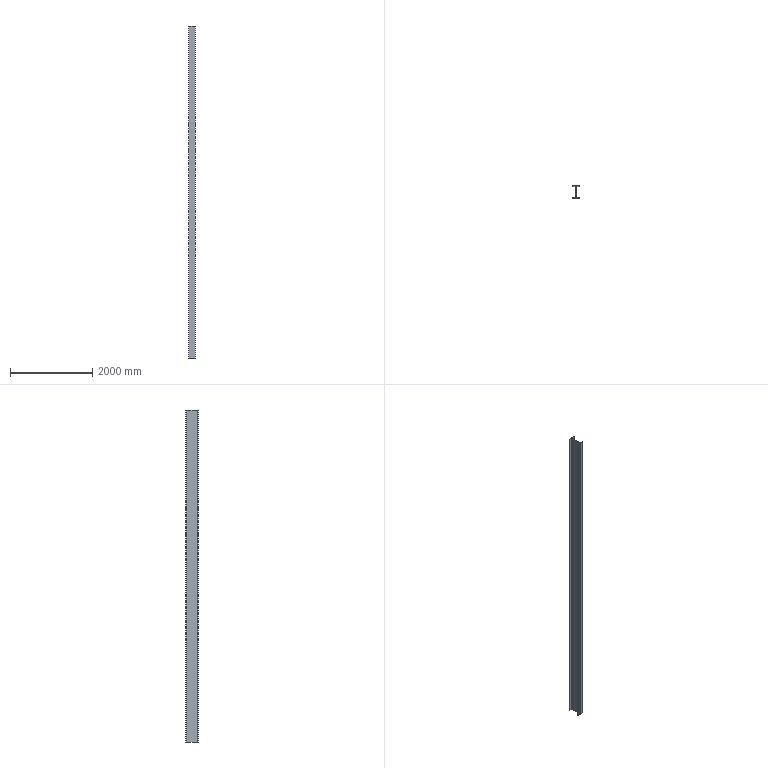Part | SolidWorks | features Extrusion 1 | 1 solid | 18 faces | box 150 x 300 x 8090 mm | volume 37845593 mm3 | plane 14 | cylinder 4 | commonest cylinder face diameters 26 x4
STEP:
#1=CARTESIAN_POINT('',(-75.,9.,0.));
#2=VERTEX_POINT('',#1);
#3=CARTESIAN_POINT('',(-75.,0.,0.));
#4=VERTEX_POINT('',#3);
#5=CARTESIAN_POINT('',(-75.,0.,0.));
#6=DIRECTION('',(0.,-1.,0.));
#7=VECTOR('',#6,1000.);
#8=LINE('',#5,#7);
#9=EDGE_CURVE('',#2,#4,#8,.T.);
#10=ORIENTED_EDGE('',*,*,#9,.T.);
#11=CARTESIAN_POINT('',(-75.,0.,8090.));
#12=VERTEX_POINT('',#11);
#13=CARTESIAN_POINT('',(-75.,0.,8090.));
#14=DIRECTION('',(0.,0.,-1.));
#15=VECTOR('',#14,1000.);
#16=LINE('',#13,#15);
#17=EDGE_CURVE('',#12,#4,#16,.T.);
#18=ORIENTED_EDGE('',*,*,#17,.F.);
#19=CARTESIAN_POINT('',(-75.,9.,8090.));
#20=VERTEX_POINT('',#19);
#21=CARTESIAN_POINT('',(-75.,0.,8090.));
#22=DIRECTION('',(0.,-1.,0.));
#23=VECTOR('',#22,1000.);
#24=LINE('',#21,#23);
#25=EDGE_CURVE('',#20,#12,#24,.T.);
#26=ORIENTED_EDGE('',*,*,#25,.F.);
#27=CARTESIAN_POINT('',(-75.,9.,8090.));
#28=DIRECTION('',(0.,0.,-1.));
#29=VECTOR('',#28,1000.);
#30=LINE('',#27,#29);
#31=EDGE_CURVE('',#20,#2,#30,.T.);
#32=ORIENTED_EDGE('',*,*,#31,.T.);
#33=EDGE_LOOP('',(#10,#18,#26,#32));
#34=FACE_OUTER_BOUND('',#33,.T.);
#35=CARTESIAN_POINT('',(-75.,0.,8090.));
#36=DIRECTION('',(1.,0.,0.));
#37=DIRECTION('',(0.,0.,-1.));
#38=AXIS2_PLACEMENT_3D('',#35,#36,#37);
#39=PLANE('',#38);
#40=ADVANCED_FACE('',(#34),#39,.F.);
#41=CARTESIAN_POINT('',(75.,0.,0.));
#42=VERTEX_POINT('',#41);
#43=CARTESIAN_POINT('',(75.,0.,0.));
#44=DIRECTION('',(1.,0.,0.));
#45=VECTOR('',#44,1000.);
#46=LINE('',#43,#45);
#47=EDGE_CURVE('',#4,#42,#46,.T.);
#48=ORIENTED_EDGE('',*,*,#47,.T.);
#49=CARTESIAN_POINT('',(75.,0.,8090.));
#50=VERTEX_POINT('',#49);
#51=CARTESIAN_POINT('',(75.,0.,8090.));
#52=DIRECTION('',(0.,0.,-1.));
#53=VECTOR('',#52,1000.);
#54=LINE('',#51,#53);
#55=EDGE_CURVE('',#50,#42,#54,.T.);
#56=ORIENTED_EDGE('',*,*,#55,.F.);
#57=CARTESIAN_POINT('',(75.,0.,8090.));
#58=DIRECTION('',(1.,0.,0.));
#59=VECTOR('',#58,1000.);
#60=LINE('',#57,#59);
#61=EDGE_CURVE('',#12,#50,#60,.T.);
#62=ORIENTED_EDGE('',*,*,#61,.F.);
#63=ORIENTED_EDGE('',*,*,#17,.T.);
#64=EDGE_LOOP('',(#48,#56,#62,#63));
#65=FACE_OUTER_BOUND('',#64,.T.);
#66=CARTESIAN_POINT('',(75.,0.,8090.));
#67=DIRECTION('',(0.,1.,0.));
#68=DIRECTION('',(-1.,0.,0.));
#69=AXIS2_PLACEMENT_3D('',#66,#67,#68);
#70=PLANE('',#69);
#71=ADVANCED_FACE('',(#65),#70,.F.);
#72=CARTESIAN_POINT('',(75.,9.,0.));
#73=VERTEX_POINT('',#72);
#74=CARTESIAN_POINT('',(75.,0.,0.));
#75=DIRECTION('',(0.,1.,0.));
#76=VECTOR('',#75,1000.);
#77=LINE('',#74,#76);
#78=EDGE_CURVE('',#42,#73,#77,.T.);
#79=ORIENTED_EDGE('',*,*,#78,.T.);
#80=CARTESIAN_POINT('',(75.,9.,8090.));
#81=VERTEX_POINT('',#80);
#82=CARTESIAN_POINT('',(75.,9.,8090.));
#83=DIRECTION('',(0.,0.,-1.));
#84=VECTOR('',#83,1000.);
#85=LINE('',#82,#84);
#86=EDGE_CURVE('',#81,#73,#85,.T.);
#87=ORIENTED_EDGE('',*,*,#86,.F.);
#88=CARTESIAN_POINT('',(75.,0.,8090.));
#89=DIRECTION('',(0.,1.,0.));
#90=VECTOR('',#89,1000.);
#91=LINE('',#88,#90);
#92=EDGE_CURVE('',#50,#81,#91,.T.);
#93=ORIENTED_EDGE('',*,*,#92,.F.);
#94=ORIENTED_EDGE('',*,*,#55,.T.);
#95=EDGE_LOOP('',(#79,#87,#93,#94));
#96=FACE_OUTER_BOUND('',#95,.T.);
#97=CARTESIAN_POINT('',(75.,0.,8090.));
#98=DIRECTION('',(-1.,0.,0.));
#99=DIRECTION('',(0.,0.,1.));
#100=AXIS2_PLACEMENT_3D('',#97,#98,#99);
#101=PLANE('',#100);
#102=ADVANCED_FACE('',(#96),#101,.F.);
#103=CARTESIAN_POINT('',(16.25,9.,0.));
#104=VERTEX_POINT('',#103);
#105=CARTESIAN_POINT('',(75.,9.,0.));
#106=DIRECTION('',(-1.,0.,0.));
#107=VECTOR('',#106,1000.);
#108=LINE('',#105,#107);
#109=EDGE_CURVE('',#73,#104,#108,.T.);
#110=ORIENTED_EDGE('',*,*,#109,.T.);
#111=CARTESIAN_POINT('',(16.25,9.,8090.));
#112=VERTEX_POINT('',#111);
#113=CARTESIAN_POINT('',(16.25,9.,8090.));
#114=DIRECTION('',(0.,0.,-1.));
#115=VECTOR('',#114,1000.);
#116=LINE('',#113,#115);
#117=EDGE_CURVE('',#112,#104,#116,.T.);
#118=ORIENTED_EDGE('',*,*,#117,.F.);
#119=CARTESIAN_POINT('',(75.,9.,8090.));
#120=DIRECTION('',(-1.,0.,0.));
#121=VECTOR('',#120,1000.);
#122=LINE('',#119,#121);
#123=EDGE_CURVE('',#81,#112,#122,.T.);
#124=ORIENTED_EDGE('',*,*,#123,.F.);
#125=ORIENTED_EDGE('',*,*,#86,.T.);
#126=EDGE_LOOP('',(#110,#118,#124,#125));
#127=FACE_OUTER_BOUND('',#126,.T.);
#128=CARTESIAN_POINT('',(75.,9.,8090.));
#129=DIRECTION('',(0.,-1.,0.));
#130=DIRECTION('',(1.,0.,0.));
#131=AXIS2_PLACEMENT_3D('',#128,#129,#130);
#132=PLANE('',#131);
#133=ADVANCED_FACE('',(#127),#132,.F.);
#134=CARTESIAN_POINT('',(3.25,22.,0.));
#135=VERTEX_POINT('',#134);
#136=CARTESIAN_POINT('',(16.25,22.,0.));
#137=DIRECTION('',(0.,0.,-1.));
#138=DIRECTION('',(-1.,0.,0.));
#139=AXIS2_PLACEMENT_3D('',#136,#137,#138);
#140=CIRCLE('',#139,13.);
#141=EDGE_CURVE('',#104,#135,#140,.T.);
#142=ORIENTED_EDGE('',*,*,#141,.T.);
#143=CARTESIAN_POINT('',(3.25,22.,8090.));
#144=VERTEX_POINT('',#143);
#145=CARTESIAN_POINT('',(3.25,22.,8090.));
#146=DIRECTION('',(0.,0.,-1.));
#147=VECTOR('',#146,1000.);
#148=LINE('',#145,#147);
#149=EDGE_CURVE('',#144,#135,#148,.T.);
#150=ORIENTED_EDGE('',*,*,#149,.F.);
#151=CARTESIAN_POINT('',(16.25,22.,8090.));
#152=DIRECTION('',(0.,0.,-1.));
#153=DIRECTION('',(-1.,0.,0.));
#154=AXIS2_PLACEMENT_3D('',#151,#152,#153);
#155=CIRCLE('',#154,13.);
#156=EDGE_CURVE('',#112,#144,#155,.T.);
#157=ORIENTED_EDGE('',*,*,#156,.F.);
#158=ORIENTED_EDGE('',*,*,#117,.T.);
#159=EDGE_LOOP('',(#142,#150,#157,#158));
#160=FACE_OUTER_BOUND('',#159,.T.);
#161=CARTESIAN_POINT('',(16.25,22.,8090.));
#162=DIRECTION('',(0.,0.,-1.));
#163=DIRECTION('',(-1.,0.,0.));
#164=AXIS2_PLACEMENT_3D('',#161,#162,#163);
#165=CYLINDRICAL_SURFACE('',#164,13.);
#166=ADVANCED_FACE('',(#160),#165,.F.);
#167=CARTESIAN_POINT('',(3.25,278.,0.));
#168=VERTEX_POINT('',#167);
#169=CARTESIAN_POINT('',(3.25,22.,0.));
#170=DIRECTION('',(0.,1.,0.));
#171=VECTOR('',#170,1000.);
#172=LINE('',#169,#171);
#173=EDGE_CURVE('',#135,#168,#172,.T.);
#174=ORIENTED_EDGE('',*,*,#173,.T.);
#175=CARTESIAN_POINT('',(3.25,278.,8090.));
#176=VERTEX_POINT('',#175);
#177=CARTESIAN_POINT('',(3.25,278.,8090.));
#178=DIRECTION('',(0.,0.,-1.));
#179=VECTOR('',#178,1000.);
#180=LINE('',#177,#179);
#181=EDGE_CURVE('',#176,#168,#180,.T.);
#182=ORIENTED_EDGE('',*,*,#181,.F.);
#183=CARTESIAN_POINT('',(3.25,22.,8090.));
#184=DIRECTION('',(0.,1.,0.));
#185=VECTOR('',#184,1000.);
#186=LINE('',#183,#185);
#187=EDGE_CURVE('',#144,#176,#186,.T.);
#188=ORIENTED_EDGE('',*,*,#187,.F.);
#189=ORIENTED_EDGE('',*,*,#149,.T.);
#190=EDGE_LOOP('',(#174,#182,#188,#189));
#191=FACE_OUTER_BOUND('',#190,.T.);
#192=CARTESIAN_POINT('',(3.25,22.,8090.));
#193=DIRECTION('',(-1.,0.,0.));
#194=DIRECTION('',(0.,0.,1.));
#195=AXIS2_PLACEMENT_3D('',#192,#193,#194);
#196=PLANE('',#195);
#197=ADVANCED_FACE('',(#191),#196,.F.);
#198=CARTESIAN_POINT('',(16.25,291.,0.));
#199=VERTEX_POINT('',#198);
#200=CARTESIAN_POINT('',(16.25,278.,0.));
#201=DIRECTION('',(0.,0.,-1.));
#202=DIRECTION('',(-1.,0.,0.));
#203=AXIS2_PLACEMENT_3D('',#200,#201,#202);
#204=CIRCLE('',#203,13.);
#205=EDGE_CURVE('',#168,#199,#204,.T.);
#206=ORIENTED_EDGE('',*,*,#205,.T.);
#207=CARTESIAN_POINT('',(16.25,291.,8090.));
#208=VERTEX_POINT('',#207);
#209=CARTESIAN_POINT('',(16.25,291.,8090.));
#210=DIRECTION('',(0.,0.,-1.));
#211=VECTOR('',#210,1000.);
#212=LINE('',#209,#211);
#213=EDGE_CURVE('',#208,#199,#212,.T.);
#214=ORIENTED_EDGE('',*,*,#213,.F.);
#215=CARTESIAN_POINT('',(16.25,278.,8090.));
#216=DIRECTION('',(0.,0.,-1.));
#217=DIRECTION('',(-1.,0.,0.));
#218=AXIS2_PLACEMENT_3D('',#215,#216,#217);
#219=CIRCLE('',#218,13.);
#220=EDGE_CURVE('',#176,#208,#219,.T.);
#221=ORIENTED_EDGE('',*,*,#220,.F.);
#222=ORIENTED_EDGE('',*,*,#181,.T.);
#223=EDGE_LOOP('',(#206,#214,#221,#222));
#224=FACE_OUTER_BOUND('',#223,.T.);
#225=CARTESIAN_POINT('',(16.25,278.,8090.));
#226=DIRECTION('',(0.,0.,-1.));
#227=DIRECTION('',(-1.,0.,0.));
#228=AXIS2_PLACEMENT_3D('',#225,#226,#227);
#229=CYLINDRICAL_SURFACE('',#228,13.);
#230=ADVANCED_FACE('',(#224),#229,.F.);
#231=CARTESIAN_POINT('',(75.,291.,0.));
#232=VERTEX_POINT('',#231);
#233=CARTESIAN_POINT('',(16.25,291.,0.));
#234=DIRECTION('',(1.,0.,0.));
#235=VECTOR('',#234,1000.);
#236=LINE('',#233,#235);
#237=EDGE_CURVE('',#199,#232,#236,.T.);
#238=ORIENTED_EDGE('',*,*,#237,.T.);
#239=CARTESIAN_POINT('',(75.,291.,8090.));
#240=VERTEX_POINT('',#239);
#241=CARTESIAN_POINT('',(75.,291.,8090.));
#242=DIRECTION('',(0.,0.,-1.));
#243=VECTOR('',#242,1000.);
#244=LINE('',#241,#243);
#245=EDGE_CURVE('',#240,#232,#244,.T.);
#246=ORIENTED_EDGE('',*,*,#245,.F.);
#247=CARTESIAN_POINT('',(16.25,291.,8090.));
#248=DIRECTION('',(1.,0.,0.));
#249=VECTOR('',#248,1000.);
#250=LINE('',#247,#249);
#251=EDGE_CURVE('',#208,#240,#250,.T.);
#252=ORIENTED_EDGE('',*,*,#251,.F.);
#253=ORIENTED_EDGE('',*,*,#213,.T.);
#254=EDGE_LOOP('',(#238,#246,#252,#253));
#255=FACE_OUTER_BOUND('',#254,.T.);
#256=CARTESIAN_POINT('',(16.25,291.,8090.));
#257=DIRECTION('',(0.,1.,0.));
#258=DIRECTION('',(-1.,0.,0.));
#259=AXIS2_PLACEMENT_3D('',#256,#257,#258);
#260=PLANE('',#259);
#261=ADVANCED_FACE('',(#255),#260,.F.);
#262=CARTESIAN_POINT('',(75.,300.,0.));
#263=VERTEX_POINT('',#262);
#264=CARTESIAN_POINT('',(75.,291.,0.));
#265=DIRECTION('',(0.,1.,0.));
#266=VECTOR('',#265,1000.);
#267=LINE('',#264,#266);
#268=EDGE_CURVE('',#232,#263,#267,.T.);
#269=ORIENTED_EDGE('',*,*,#268,.T.);
#270=CARTESIAN_POINT('',(75.,300.,8090.));
#271=VERTEX_POINT('',#270);
#272=CARTESIAN_POINT('',(75.,300.,8090.));
#273=DIRECTION('',(0.,0.,-1.));
#274=VECTOR('',#273,1000.);
#275=LINE('',#272,#274);
#276=EDGE_CURVE('',#271,#263,#275,.T.);
#277=ORIENTED_EDGE('',*,*,#276,.F.);
#278=CARTESIAN_POINT('',(75.,291.,8090.));
#279=DIRECTION('',(0.,1.,0.));
#280=VECTOR('',#279,1000.);
#281=LINE('',#278,#280);
#282=EDGE_CURVE('',#240,#271,#281,.T.);
#283=ORIENTED_EDGE('',*,*,#282,.F.);
#284=ORIENTED_EDGE('',*,*,#245,.T.);
#285=EDGE_LOOP('',(#269,#277,#283,#284));
#286=FACE_OUTER_BOUND('',#285,.T.);
#287=CARTESIAN_POINT('',(75.,291.,8090.));
#288=DIRECTION('',(-1.,0.,0.));
#289=DIRECTION('',(0.,-1.,0.));
#290=AXIS2_PLACEMENT_3D('',#287,#288,#289);
#291=PLANE('',#290);
#292=ADVANCED_FACE('',(#286),#291,.F.);
#293=CARTESIAN_POINT('',(-75.,300.,0.));
#294=VERTEX_POINT('',#293);
#295=CARTESIAN_POINT('',(-75.,300.,0.));
#296=DIRECTION('',(-1.,0.,0.));
#297=VECTOR('',#296,1000.);
#298=LINE('',#295,#297);
#299=EDGE_CURVE('',#263,#294,#298,.T.);
#300=ORIENTED_EDGE('',*,*,#299,.T.);
#301=CARTESIAN_POINT('',(-75.,300.,8090.));
#302=VERTEX_POINT('',#301);
#303=CARTESIAN_POINT('',(-75.,300.,8090.));
#304=DIRECTION('',(0.,0.,-1.));
#305=VECTOR('',#304,1000.);
#306=LINE('',#303,#305);
#307=EDGE_CURVE('',#302,#294,#306,.T.);
#308=ORIENTED_EDGE('',*,*,#307,.F.);
#309=CARTESIAN_POINT('',(-75.,300.,8090.));
#310=DIRECTION('',(-1.,0.,0.));
#311=VECTOR('',#310,1000.);
#312=LINE('',#309,#311);
#313=EDGE_CURVE('',#271,#302,#312,.T.);
#314=ORIENTED_EDGE('',*,*,#313,.F.);
#315=ORIENTED_EDGE('',*,*,#276,.T.);
#316=EDGE_LOOP('',(#300,#308,#314,#315));
#317=FACE_OUTER_BOUND('',#316,.T.);
#318=CARTESIAN_POINT('',(-75.,300.,8090.));
#319=DIRECTION('',(0.,-1.,0.));
#320=DIRECTION('',(0.,0.,-1.));
#321=AXIS2_PLACEMENT_3D('',#318,#319,#320);
#322=PLANE('',#321);
#323=ADVANCED_FACE('',(#317),#322,.F.);
#324=CARTESIAN_POINT('',(-75.,291.,0.));
#325=VERTEX_POINT('',#324);
#326=CARTESIAN_POINT('',(-75.,291.,0.));
#327=DIRECTION('',(0.,-1.,0.));
#328=VECTOR('',#327,1000.);
#329=LINE('',#326,#328);
#330=EDGE_CURVE('',#294,#325,#329,.T.);
#331=ORIENTED_EDGE('',*,*,#330,.T.);
#332=CARTESIAN_POINT('',(-75.,291.,8090.));
#333=VERTEX_POINT('',#332);
#334=CARTESIAN_POINT('',(-75.,291.,8090.));
#335=DIRECTION('',(0.,0.,-1.));
#336=VECTOR('',#335,1000.);
#337=LINE('',#334,#336);
#338=EDGE_CURVE('',#333,#325,#337,.T.);
#339=ORIENTED_EDGE('',*,*,#338,.F.);
#340=CARTESIAN_POINT('',(-75.,291.,8090.));
#341=DIRECTION('',(0.,-1.,0.));
#342=VECTOR('',#341,1000.);
#343=LINE('',#340,#342);
#344=EDGE_CURVE('',#302,#333,#343,.T.);
#345=ORIENTED_EDGE('',*,*,#344,.F.);
#346=ORIENTED_EDGE('',*,*,#307,.T.);
#347=EDGE_LOOP('',(#331,#339,#345,#346));
#348=FACE_OUTER_BOUND('',#347,.T.);
#349=CARTESIAN_POINT('',(-75.,291.,8090.));
#350=DIRECTION('',(1.,0.,0.));
#351=DIRECTION('',(0.,1.,0.));
#352=AXIS2_PLACEMENT_3D('',#349,#350,#351);
#353=PLANE('',#352);
#354=ADVANCED_FACE('',(#348),#353,.F.);
#355=CARTESIAN_POINT('',(-16.25,291.,0.));
#356=VERTEX_POINT('',#355);
#357=CARTESIAN_POINT('',(-16.25,291.,0.));
#358=DIRECTION('',(1.,0.,0.));
#359=VECTOR('',#358,1000.);
#360=LINE('',#357,#359);
#361=EDGE_CURVE('',#325,#356,#360,.T.);
#362=ORIENTED_EDGE('',*,*,#361,.T.);
#363=CARTESIAN_POINT('',(-16.25,291.,8090.));
#364=VERTEX_POINT('',#363);
#365=CARTESIAN_POINT('',(-16.25,291.,8090.));
#366=DIRECTION('',(0.,0.,-1.));
#367=VECTOR('',#366,1000.);
#368=LINE('',#365,#367);
#369=EDGE_CURVE('',#364,#356,#368,.T.);
#370=ORIENTED_EDGE('',*,*,#369,.F.);
#371=CARTESIAN_POINT('',(-16.25,291.,8090.));
#372=DIRECTION('',(1.,0.,0.));
#373=VECTOR('',#372,1000.);
#374=LINE('',#371,#373);
#375=EDGE_CURVE('',#333,#364,#374,.T.);
#376=ORIENTED_EDGE('',*,*,#375,.F.);
#377=ORIENTED_EDGE('',*,*,#338,.T.);
#378=EDGE_LOOP('',(#362,#370,#376,#377));
#379=FACE_OUTER_BOUND('',#378,.T.);
#380=CARTESIAN_POINT('',(-16.25,291.,8090.));
#381=DIRECTION('',(0.,1.,0.));
#382=DIRECTION('',(-1.,0.,0.));
#383=AXIS2_PLACEMENT_3D('',#380,#381,#382);
#384=PLANE('',#383);
#385=ADVANCED_FACE('',(#379),#384,.F.);
#386=CARTESIAN_POINT('',(-3.25,278.,0.));
#387=VERTEX_POINT('',#386);
#388=CARTESIAN_POINT('',(-16.25,278.,0.));
#389=DIRECTION('',(0.,0.,-1.));
#390=DIRECTION('',(1.,0.,0.));
#391=AXIS2_PLACEMENT_3D('',#388,#389,#390);
#392=CIRCLE('',#391,13.);
#393=EDGE_CURVE('',#356,#387,#392,.T.);
#394=ORIENTED_EDGE('',*,*,#393,.T.);
#395=CARTESIAN_POINT('',(-3.25,278.,8090.));
#396=VERTEX_POINT('',#395);
#397=CARTESIAN_POINT('',(-3.25,278.,8090.));
#398=DIRECTION('',(0.,0.,-1.));
#399=VECTOR('',#398,1000.);
#400=LINE('',#397,#399);
#401=EDGE_CURVE('',#396,#387,#400,.T.);
#402=ORIENTED_EDGE('',*,*,#401,.F.);
#403=CARTESIAN_POINT('',(-16.25,278.,8090.));
#404=DIRECTION('',(0.,0.,-1.));
#405=DIRECTION('',(1.,0.,0.));
#406=AXIS2_PLACEMENT_3D('',#403,#404,#405);
#407=CIRCLE('',#406,13.);
#408=EDGE_CURVE('',#364,#396,#407,.T.);
#409=ORIENTED_EDGE('',*,*,#408,.F.);
#410=ORIENTED_EDGE('',*,*,#369,.T.);
#411=EDGE_LOOP('',(#394,#402,#409,#410));
#412=FACE_OUTER_BOUND('',#411,.T.);
#413=CARTESIAN_POINT('',(-16.25,278.,8090.));
#414=DIRECTION('',(0.,0.,-1.));
#415=DIRECTION('',(-1.,0.,0.));
#416=AXIS2_PLACEMENT_3D('',#413,#414,#415);
#417=CYLINDRICAL_SURFACE('',#416,13.);
#418=ADVANCED_FACE('',(#412),#417,.F.);
#419=CARTESIAN_POINT('',(-3.25,22.,0.));
#420=VERTEX_POINT('',#419);
#421=CARTESIAN_POINT('',(-3.25,22.,0.));
#422=DIRECTION('',(0.,-1.,0.));
#423=VECTOR('',#422,1000.);
#424=LINE('',#421,#423);
#425=EDGE_CURVE('',#387,#420,#424,.T.);
#426=ORIENTED_EDGE('',*,*,#425,.T.);
#427=CARTESIAN_POINT('',(-3.25,22.,8090.));
#428=VERTEX_POINT('',#427);
#429=CARTESIAN_POINT('',(-3.25,22.,8090.));
#430=DIRECTION('',(0.,0.,-1.));
#431=VECTOR('',#430,1000.);
#432=LINE('',#429,#431);
#433=EDGE_CURVE('',#428,#420,#432,.T.);
#434=ORIENTED_EDGE('',*,*,#433,.F.);
#435=CARTESIAN_POINT('',(-3.25,22.,8090.));
#436=DIRECTION('',(0.,-1.,0.));
#437=VECTOR('',#436,1000.);
#438=LINE('',#435,#437);
#439=EDGE_CURVE('',#396,#428,#438,.T.);
#440=ORIENTED_EDGE('',*,*,#439,.F.);
#441=ORIENTED_EDGE('',*,*,#401,.T.);
#442=EDGE_LOOP('',(#426,#434,#440,#441));
#443=FACE_OUTER_BOUND('',#442,.T.);
#444=CARTESIAN_POINT('',(-3.25,22.,8090.));
#445=DIRECTION('',(1.,0.,0.));
#446=DIRECTION('',(0.,0.,-1.));
#447=AXIS2_PLACEMENT_3D('',#444,#445,#446);
#448=PLANE('',#447);
#449=ADVANCED_FACE('',(#443),#448,.F.);
#450=CARTESIAN_POINT('',(-16.25,9.,0.));
#451=VERTEX_POINT('',#450);
#452=CARTESIAN_POINT('',(-16.25,22.,0.));
#453=DIRECTION('',(0.,0.,-1.));
#454=DIRECTION('',(-1.,0.,0.));
#455=AXIS2_PLACEMENT_3D('',#452,#453,#454);
#456=CIRCLE('',#455,13.);
#457=EDGE_CURVE('',#420,#451,#456,.T.);
#458=ORIENTED_EDGE('',*,*,#457,.T.);
#459=CARTESIAN_POINT('',(-16.25,9.,8090.));
#460=VERTEX_POINT('',#459);
#461=CARTESIAN_POINT('',(-16.25,9.,8090.));
#462=DIRECTION('',(0.,0.,-1.));
#463=VECTOR('',#462,1000.);
#464=LINE('',#461,#463);
#465=EDGE_CURVE('',#460,#451,#464,.T.);
#466=ORIENTED_EDGE('',*,*,#465,.F.);
#467=CARTESIAN_POINT('',(-16.25,22.,8090.));
#468=DIRECTION('',(0.,0.,-1.));
#469=DIRECTION('',(-1.,0.,0.));
#470=AXIS2_PLACEMENT_3D('',#467,#468,#469);
#471=CIRCLE('',#470,13.);
#472=EDGE_CURVE('',#428,#460,#471,.T.);
#473=ORIENTED_EDGE('',*,*,#472,.F.);
#474=ORIENTED_EDGE('',*,*,#433,.T.);
#475=EDGE_LOOP('',(#458,#466,#473,#474));
#476=FACE_OUTER_BOUND('',#475,.T.);
#477=CARTESIAN_POINT('',(-16.25,22.,8090.));
#478=DIRECTION('',(0.,0.,-1.));
#479=DIRECTION('',(-1.,0.,0.));
#480=AXIS2_PLACEMENT_3D('',#477,#478,#479);
#481=CYLINDRICAL_SURFACE('',#480,13.);
#482=ADVANCED_FACE('',(#476),#481,.F.);
#483=CARTESIAN_POINT('',(-75.,9.,0.));
#484=DIRECTION('',(-1.,0.,0.));
#485=VECTOR('',#484,1000.);
#486=LINE('',#483,#485);
#487=EDGE_CURVE('',#451,#2,#486,.T.);
#488=ORIENTED_EDGE('',*,*,#487,.T.);
#489=ORIENTED_EDGE('',*,*,#31,.F.);
#490=CARTESIAN_POINT('',(-75.,9.,8090.));
#491=DIRECTION('',(-1.,0.,0.));
#492=VECTOR('',#491,1000.);
#493=LINE('',#490,#492);
#494=EDGE_CURVE('',#460,#20,#493,.T.);
#495=ORIENTED_EDGE('',*,*,#494,.F.);
#496=ORIENTED_EDGE('',*,*,#465,.T.);
#497=EDGE_LOOP('',(#488,#489,#495,#496));
#498=FACE_OUTER_BOUND('',#497,.T.);
#499=CARTESIAN_POINT('',(-75.,9.,8090.));
#500=DIRECTION('',(0.,-1.,0.));
#501=DIRECTION('',(1.,0.,0.));
#502=AXIS2_PLACEMENT_3D('',#499,#500,#501);
#503=PLANE('',#502);
#504=ADVANCED_FACE('',(#498),#503,.F.);
#505=ORIENTED_EDGE('',*,*,#25,.T.);
#506=ORIENTED_EDGE('',*,*,#61,.T.);
#507=ORIENTED_EDGE('',*,*,#92,.T.);
#508=ORIENTED_EDGE('',*,*,#123,.T.);
#509=ORIENTED_EDGE('',*,*,#156,.T.);
#510=ORIENTED_EDGE('',*,*,#187,.T.);
#511=ORIENTED_EDGE('',*,*,#220,.T.);
#512=ORIENTED_EDGE('',*,*,#251,.T.);
#513=ORIENTED_EDGE('',*,*,#282,.T.);
#514=ORIENTED_EDGE('',*,*,#313,.T.);
#515=ORIENTED_EDGE('',*,*,#344,.T.);
#516=ORIENTED_EDGE('',*,*,#375,.T.);
#517=ORIENTED_EDGE('',*,*,#408,.T.);
#518=ORIENTED_EDGE('',*,*,#439,.T.);
#519=ORIENTED_EDGE('',*,*,#472,.T.);
#520=ORIENTED_EDGE('',*,*,#494,.T.);
#521=EDGE_LOOP('',(#505,#506,#507,#508,#509,#510,#511,#512,#513,#514,#515,#516,#517,#518,#519,#520));
#522=FACE_OUTER_BOUND('',#521,.T.);
#523=CARTESIAN_POINT('',(-16.25,22.,8090.));
#524=DIRECTION('',(0.,0.,-1.));
#525=DIRECTION('',(-1.,0.,0.));
#526=AXIS2_PLACEMENT_3D('',#523,#524,#525);
#527=PLANE('',#526);
#528=ADVANCED_FACE('',(#522),#527,.F.);
#529=ORIENTED_EDGE('',*,*,#9,.F.);
#530=ORIENTED_EDGE('',*,*,#487,.F.);
#531=ORIENTED_EDGE('',*,*,#457,.F.);
#532=ORIENTED_EDGE('',*,*,#425,.F.);
#533=ORIENTED_EDGE('',*,*,#393,.F.);
#534=ORIENTED_EDGE('',*,*,#361,.F.);
#535=ORIENTED_EDGE('',*,*,#330,.F.);
#536=ORIENTED_EDGE('',*,*,#299,.F.);
#537=ORIENTED_EDGE('',*,*,#268,.F.);
#538=ORIENTED_EDGE('',*,*,#237,.F.);
#539=ORIENTED_EDGE('',*,*,#205,.F.);
#540=ORIENTED_EDGE('',*,*,#173,.F.);
#541=ORIENTED_EDGE('',*,*,#141,.F.);
#542=ORIENTED_EDGE('',*,*,#109,.F.);
#543=ORIENTED_EDGE('',*,*,#78,.F.);
#544=ORIENTED_EDGE('',*,*,#47,.F.);
#545=EDGE_LOOP('',(#529,#530,#531,#532,#533,#534,#535,#536,#537,#538,#539,#540,#541,#542,#543,#544));
#546=FACE_OUTER_BOUND('',#545,.T.);
#547=CARTESIAN_POINT('',(-16.25,22.,0.));
#548=DIRECTION('',(0.,0.,-1.));
#549=DIRECTION('',(-1.,0.,0.));
#550=AXIS2_PLACEMENT_3D('',#547,#548,#549);
#551=PLANE('',#550);
#552=ADVANCED_FACE('',(#546),#551,.T.);
#553=CLOSED_SHELL('',(#40,#71,#102,#133,#166,#197,#230,#261,#292,#323,#354,#385,#418,#449,#482,#504,#528,#552));
#554=MANIFOLD_SOLID_BREP('',#553);
#555=CARTESIAN_POINT('',(0.,0.,0.));
#556=DIRECTION('',(0.,0.,1.));
#557=DIRECTION('',(1.,0.,0.));
#558=AXIS2_PLACEMENT_3D('',#555,#556,#557);
#559=(LENGTH_UNIT()NAMED_UNIT(*)SI_UNIT(.MILLI.,.METRE.));
#560=UNCERTAINTY_MEASURE_WITH_UNIT(LENGTH_MEASURE(0.00001),#559,'','');
#561=(NAMED_UNIT(*)PLANE_ANGLE_UNIT()SI_UNIT($,.RADIAN.));
#562=(NAMED_UNIT(*)SI_UNIT($,.STERADIAN.)SOLID_ANGLE_UNIT());
#563=(GEOMETRIC_REPRESENTATION_CONTEXT(3)GLOBAL_UNCERTAINTY_ASSIGNED_CONTEXT((#560))GLOBAL_UNIT_ASSIGNED_CONTEXT((#559,#561,#562))REPRESENTATION_CONTEXT('',''));
#564=ADVANCED_BREP_SHAPE_REPRESENTATION('',(#554,#558),#563);